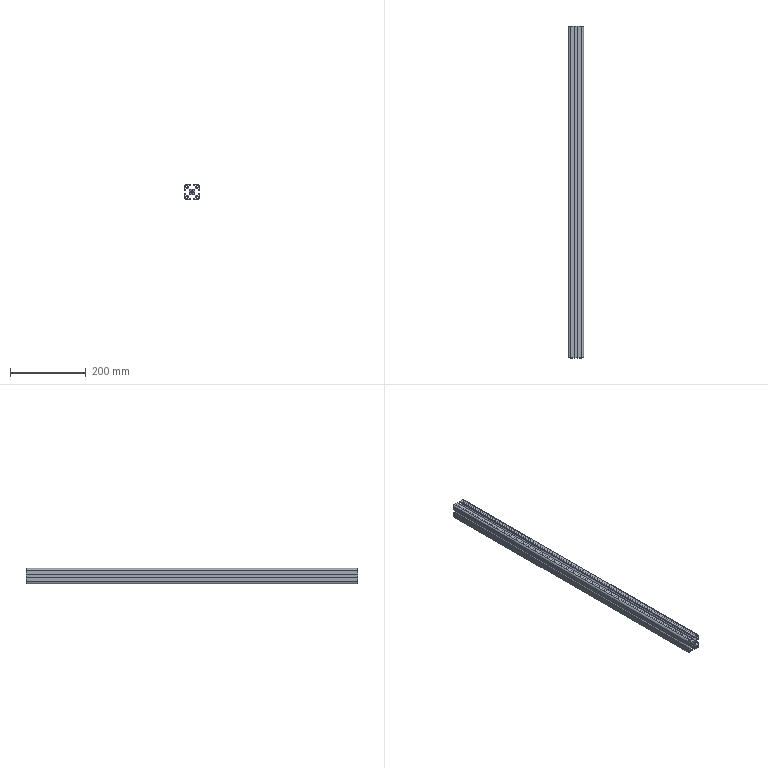Part | 1 solid | 104 faces | box 40 x 876 x 40 mm | volume 505054 mm3 | plane 94 | cylinder 10 | commonest cylinder face diameters 5 x4 9 x4 6.8 x2